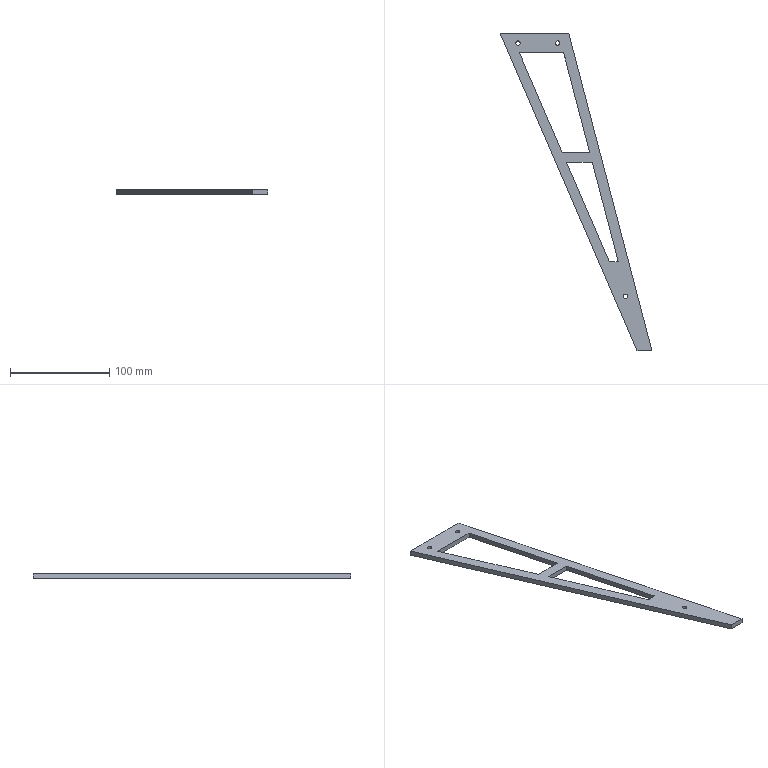Part | SolidWorks | features ICE 3, Extrusion 1 | 1 solid | 20 faces | box 152.846 x 320 x 5 mm | volume 40320 mm3 | plane 14 | cylinder 6 | commonest cylinder face diameters 4.4 x6
STEP:
#1=CARTESIAN_POINT('',(226.262,-608.,-2.5));
#2=VERTEX_POINT('',#1);
#3=CARTESIAN_POINT('',(230.662,-608.,-2.5));
#4=VERTEX_POINT('',#3);
#5=CARTESIAN_POINT('',(228.462,-608.,-2.5));
#6=DIRECTION('',(0.,0.,1.));
#7=DIRECTION('',(1.,0.,0.));
#8=AXIS2_PLACEMENT_3D('',#5,#6,#7);
#9=CIRCLE('',#8,2.2);
#10=EDGE_CURVE('',#2,#4,#9,.T.);
#11=ORIENTED_EDGE('',*,*,#10,.F.);
#12=CARTESIAN_POINT('',(226.262,-608.,2.5));
#13=VERTEX_POINT('',#12);
#14=CARTESIAN_POINT('',(226.262,-608.,-7.5));
#15=DIRECTION('',(0.,0.,1.));
#16=VECTOR('',#15,1000.);
#17=LINE('',#14,#16);
#18=EDGE_CURVE('',#2,#13,#17,.T.);
#19=ORIENTED_EDGE('',*,*,#18,.T.);
#20=CARTESIAN_POINT('',(230.662,-608.,2.5));
#21=VERTEX_POINT('',#20);
#22=CARTESIAN_POINT('',(228.462,-608.,2.5));
#23=DIRECTION('',(0.,0.,1.));
#24=DIRECTION('',(1.,0.,0.));
#25=AXIS2_PLACEMENT_3D('',#22,#23,#24);
#26=CIRCLE('',#25,2.2);
#27=EDGE_CURVE('',#13,#21,#26,.T.);
#28=ORIENTED_EDGE('',*,*,#27,.T.);
#29=CARTESIAN_POINT('',(230.662,-608.,-7.5));
#30=DIRECTION('',(0.,0.,1.));
#31=VECTOR('',#30,1000.);
#32=LINE('',#29,#31);
#33=EDGE_CURVE('',#4,#21,#32,.T.);
#34=ORIENTED_EDGE('',*,*,#33,.F.);
#35=EDGE_LOOP('',(#11,#19,#28,#34));
#36=FACE_OUTER_BOUND('',#35,.T.);
#37=CARTESIAN_POINT('',(228.462,-608.,-7.5));
#38=DIRECTION('',(0.,0.,1.));
#39=DIRECTION('',(1.,0.,0.));
#40=AXIS2_PLACEMENT_3D('',#37,#38,#39);
#41=CYLINDRICAL_SURFACE('',#40,2.2);
#42=ADVANCED_FACE('',(#36),#41,.F.);
#43=CARTESIAN_POINT('',(117.992,-353.,-2.5));
#44=VERTEX_POINT('',#43);
#45=CARTESIAN_POINT('',(122.392,-353.,-2.5));
#46=VERTEX_POINT('',#45);
#47=CARTESIAN_POINT('',(120.192,-353.,-2.5));
#48=DIRECTION('',(0.,0.,1.));
#49=DIRECTION('',(1.,0.,0.));
#50=AXIS2_PLACEMENT_3D('',#47,#48,#49);
#51=CIRCLE('',#50,2.2);
#52=EDGE_CURVE('',#44,#46,#51,.T.);
#53=ORIENTED_EDGE('',*,*,#52,.F.);
#54=CARTESIAN_POINT('',(117.992,-353.,2.5));
#55=VERTEX_POINT('',#54);
#56=CARTESIAN_POINT('',(117.992,-353.,-7.5));
#57=DIRECTION('',(0.,0.,1.));
#58=VECTOR('',#57,1000.);
#59=LINE('',#56,#58);
#60=EDGE_CURVE('',#44,#55,#59,.T.);
#61=ORIENTED_EDGE('',*,*,#60,.T.);
#62=CARTESIAN_POINT('',(122.392,-353.,2.5));
#63=VERTEX_POINT('',#62);
#64=CARTESIAN_POINT('',(120.192,-353.,2.5));
#65=DIRECTION('',(0.,0.,1.));
#66=DIRECTION('',(1.,0.,0.));
#67=AXIS2_PLACEMENT_3D('',#64,#65,#66);
#68=CIRCLE('',#67,2.2);
#69=EDGE_CURVE('',#55,#63,#68,.T.);
#70=ORIENTED_EDGE('',*,*,#69,.T.);
#71=CARTESIAN_POINT('',(122.392,-353.,-7.5));
#72=DIRECTION('',(0.,0.,1.));
#73=VECTOR('',#72,1000.);
#74=LINE('',#71,#73);
#75=EDGE_CURVE('',#46,#63,#74,.T.);
#76=ORIENTED_EDGE('',*,*,#75,.F.);
#77=EDGE_LOOP('',(#53,#61,#70,#76));
#78=FACE_OUTER_BOUND('',#77,.T.);
#79=CARTESIAN_POINT('',(120.192,-353.,-7.5));
#80=DIRECTION('',(0.,0.,1.));
#81=DIRECTION('',(1.,0.,0.));
#82=AXIS2_PLACEMENT_3D('',#79,#80,#81);
#83=CYLINDRICAL_SURFACE('',#82,2.2);
#84=ADVANCED_FACE('',(#78),#83,.F.);
#85=CARTESIAN_POINT('',(157.992,-353.,-2.5));
#86=VERTEX_POINT('',#85);
#87=CARTESIAN_POINT('',(162.392,-353.,-2.5));
#88=VERTEX_POINT('',#87);
#89=CARTESIAN_POINT('',(160.192,-353.,-2.5));
#90=DIRECTION('',(0.,0.,1.));
#91=DIRECTION('',(1.,0.,0.));
#92=AXIS2_PLACEMENT_3D('',#89,#90,#91);
#93=CIRCLE('',#92,2.2);
#94=EDGE_CURVE('',#86,#88,#93,.T.);
#95=ORIENTED_EDGE('',*,*,#94,.F.);
#96=CARTESIAN_POINT('',(157.992,-353.,2.5));
#97=VERTEX_POINT('',#96);
#98=CARTESIAN_POINT('',(157.992,-353.,-7.5));
#99=DIRECTION('',(0.,0.,1.));
#100=VECTOR('',#99,1000.);
#101=LINE('',#98,#100);
#102=EDGE_CURVE('',#86,#97,#101,.T.);
#103=ORIENTED_EDGE('',*,*,#102,.T.);
#104=CARTESIAN_POINT('',(162.392,-353.,2.5));
#105=VERTEX_POINT('',#104);
#106=CARTESIAN_POINT('',(160.192,-353.,2.5));
#107=DIRECTION('',(0.,0.,1.));
#108=DIRECTION('',(1.,0.,0.));
#109=AXIS2_PLACEMENT_3D('',#106,#107,#108);
#110=CIRCLE('',#109,2.2);
#111=EDGE_CURVE('',#97,#105,#110,.T.);
#112=ORIENTED_EDGE('',*,*,#111,.T.);
#113=CARTESIAN_POINT('',(162.392,-353.,-7.5));
#114=DIRECTION('',(0.,0.,1.));
#115=VECTOR('',#114,1000.);
#116=LINE('',#113,#115);
#117=EDGE_CURVE('',#88,#105,#116,.T.);
#118=ORIENTED_EDGE('',*,*,#117,.F.);
#119=EDGE_LOOP('',(#95,#103,#112,#118));
#120=FACE_OUTER_BOUND('',#119,.T.);
#121=CARTESIAN_POINT('',(160.192,-353.,-7.5));
#122=DIRECTION('',(0.,0.,1.));
#123=DIRECTION('',(1.,0.,0.));
#124=AXIS2_PLACEMENT_3D('',#121,#122,#123);
#125=CYLINDRICAL_SURFACE('',#124,2.2);
#126=ADVANCED_FACE('',(#120),#125,.F.);
#127=CARTESIAN_POINT('',(102.154,-343.,-2.5));
#128=VERTEX_POINT('',#127);
#129=CARTESIAN_POINT('',(171.308,-343.,-2.5));
#130=VERTEX_POINT('',#129);
#131=CARTESIAN_POINT('',(0.,-343.,-2.5));
#132=DIRECTION('',(1.,0.,0.));
#133=VECTOR('',#132,1000.);
#134=LINE('',#131,#133);
#135=EDGE_CURVE('',#128,#130,#134,.T.);
#136=ORIENTED_EDGE('',*,*,#135,.F.);
#137=CARTESIAN_POINT('',(102.154,-343.,2.5));
#138=VERTEX_POINT('',#137);
#139=CARTESIAN_POINT('',(102.154,-343.,2.5));
#140=DIRECTION('',(0.,0.,-1.));
#141=VECTOR('',#140,1000.);
#142=LINE('',#139,#141);
#143=EDGE_CURVE('',#138,#128,#142,.T.);
#144=ORIENTED_EDGE('',*,*,#143,.F.);
#145=CARTESIAN_POINT('',(171.308,-343.,2.5));
#146=VERTEX_POINT('',#145);
#147=CARTESIAN_POINT('',(0.,-343.,2.5));
#148=DIRECTION('',(1.,0.,0.));
#149=VECTOR('',#148,1000.);
#150=LINE('',#147,#149);
#151=EDGE_CURVE('',#138,#146,#150,.T.);
#152=ORIENTED_EDGE('',*,*,#151,.T.);
#153=CARTESIAN_POINT('',(171.308,-343.,2.5));
#154=DIRECTION('',(0.,0.,-1.));
#155=VECTOR('',#154,1000.);
#156=LINE('',#153,#155);
#157=EDGE_CURVE('',#146,#130,#156,.T.);
#158=ORIENTED_EDGE('',*,*,#157,.T.);
#159=EDGE_LOOP('',(#136,#144,#152,#158));
#160=FACE_OUTER_BOUND('',#159,.T.);
#161=CARTESIAN_POINT('',(0.,-343.,2.5));
#162=DIRECTION('',(0.,1.,0.));
#163=DIRECTION('',(0.,0.,1.));
#164=AXIS2_PLACEMENT_3D('',#161,#162,#163);
#165=PLANE('',#164);
#166=ADVANCED_FACE('',(#160),#165,.T.);
#167=CARTESIAN_POINT('',(240.,-663.,-2.5));
#168=VERTEX_POINT('',#167);
#169=CARTESIAN_POINT('',(-38.463,-16.569,-2.5));
#170=DIRECTION('',(-0.3956,0.9184,0.));
#171=VECTOR('',#170,1000.);
#172=LINE('',#169,#171);
#173=EDGE_CURVE('',#168,#128,#172,.T.);
#174=ORIENTED_EDGE('',*,*,#173,.F.);
#175=CARTESIAN_POINT('',(240.,-663.,2.5));
#176=VERTEX_POINT('',#175);
#177=CARTESIAN_POINT('',(240.,-663.,2.5));
#178=DIRECTION('',(0.,0.,-1.));
#179=VECTOR('',#178,1000.);
#180=LINE('',#177,#179);
#181=EDGE_CURVE('',#176,#168,#180,.T.);
#182=ORIENTED_EDGE('',*,*,#181,.F.);
#183=CARTESIAN_POINT('',(-38.463,-16.569,2.5));
#184=DIRECTION('',(-0.3956,0.9184,0.));
#185=VECTOR('',#184,1000.);
#186=LINE('',#183,#185);
#187=EDGE_CURVE('',#176,#138,#186,.T.);
#188=ORIENTED_EDGE('',*,*,#187,.T.);
#189=ORIENTED_EDGE('',*,*,#143,.T.);
#190=EDGE_LOOP('',(#174,#182,#188,#189));
#191=FACE_OUTER_BOUND('',#190,.T.);
#192=CARTESIAN_POINT('',(-38.463,-16.569,2.5));
#193=DIRECTION('',(-0.9184,-0.3956,0.));
#194=DIRECTION('',(0.3956,-0.9184,0.));
#195=AXIS2_PLACEMENT_3D('',#192,#193,#194);
#196=PLANE('',#195);
#197=ADVANCED_FACE('',(#191),#196,.T.);
#198=CARTESIAN_POINT('',(255.,-663.,-2.5));
#199=VERTEX_POINT('',#198);
#200=CARTESIAN_POINT('',(0.,-663.,-2.5));
#201=DIRECTION('',(-1.,0.,0.));
#202=VECTOR('',#201,1000.);
#203=LINE('',#200,#202);
#204=EDGE_CURVE('',#199,#168,#203,.T.);
#205=ORIENTED_EDGE('',*,*,#204,.F.);
#206=CARTESIAN_POINT('',(255.,-663.,2.5));
#207=VERTEX_POINT('',#206);
#208=CARTESIAN_POINT('',(255.,-663.,2.5));
#209=DIRECTION('',(0.,0.,-1.));
#210=VECTOR('',#209,1000.);
#211=LINE('',#208,#210);
#212=EDGE_CURVE('',#207,#199,#211,.T.);
#213=ORIENTED_EDGE('',*,*,#212,.F.);
#214=CARTESIAN_POINT('',(0.,-663.,2.5));
#215=DIRECTION('',(-1.,0.,0.));
#216=VECTOR('',#215,1000.);
#217=LINE('',#214,#216);
#218=EDGE_CURVE('',#207,#176,#217,.T.);
#219=ORIENTED_EDGE('',*,*,#218,.T.);
#220=ORIENTED_EDGE('',*,*,#181,.T.);
#221=EDGE_LOOP('',(#205,#213,#219,#220));
#222=FACE_OUTER_BOUND('',#221,.T.);
#223=CARTESIAN_POINT('',(0.,-663.,2.5));
#224=DIRECTION('',(0.,-1.,0.));
#225=DIRECTION('',(1.,0.,0.));
#226=AXIS2_PLACEMENT_3D('',#223,#224,#225);
#227=PLANE('',#226);
#228=ADVANCED_FACE('',(#222),#227,.T.);
#229=CARTESIAN_POINT('',(76.376,19.975,-2.5));
#230=DIRECTION('',(0.253,-0.9675,0.));
#231=VECTOR('',#230,1000.);
#232=LINE('',#229,#231);
#233=EDGE_CURVE('',#130,#199,#232,.T.);
#234=ORIENTED_EDGE('',*,*,#233,.F.);
#235=ORIENTED_EDGE('',*,*,#157,.F.);
#236=CARTESIAN_POINT('',(76.376,19.975,2.5));
#237=DIRECTION('',(0.253,-0.9675,0.));
#238=VECTOR('',#237,1000.);
#239=LINE('',#236,#238);
#240=EDGE_CURVE('',#146,#207,#239,.T.);
#241=ORIENTED_EDGE('',*,*,#240,.T.);
#242=ORIENTED_EDGE('',*,*,#212,.T.);
#243=EDGE_LOOP('',(#234,#235,#241,#242));
#244=FACE_OUTER_BOUND('',#243,.T.);
#245=CARTESIAN_POINT('',(76.376,19.975,2.5));
#246=DIRECTION('',(0.9675,0.253,0.));
#247=DIRECTION('',(-0.253,0.9675,0.));
#248=AXIS2_PLACEMENT_3D('',#245,#246,#247);
#249=PLANE('',#248);
#250=ADVANCED_FACE('',(#244),#249,.T.);
#251=CARTESIAN_POINT('',(228.462,-608.,2.5));
#252=DIRECTION('',(0.,0.,1.));
#253=DIRECTION('',(1.,0.,0.));
#254=AXIS2_PLACEMENT_3D('',#251,#252,#253);
#255=CIRCLE('',#254,2.2);
#256=EDGE_CURVE('',#21,#13,#255,.T.);
#257=ORIENTED_EDGE('',*,*,#256,.F.);
#258=ORIENTED_EDGE('',*,*,#27,.F.);
#259=EDGE_LOOP('',(#257,#258));
#260=FACE_BOUND('',#259,.T.);
#261=CARTESIAN_POINT('',(164.735,-463.,2.5));
#262=VERTEX_POINT('',#261);
#263=CARTESIAN_POINT('',(192.356,-463.,2.5));
#264=VERTEX_POINT('',#263);
#265=CARTESIAN_POINT('',(0.,-463.,2.5));
#266=DIRECTION('',(1.,0.,0.));
#267=VECTOR('',#266,1000.);
#268=LINE('',#265,#267);
#269=EDGE_CURVE('',#262,#264,#268,.T.);
#270=ORIENTED_EDGE('',*,*,#269,.F.);
#271=CARTESIAN_POINT('',(121.658,-363.,2.5));
#272=VERTEX_POINT('',#271);
#273=CARTESIAN_POINT('',(-29.279,-12.612,2.5));
#274=DIRECTION('',(0.3956,-0.9184,0.));
#275=VECTOR('',#274,1000.);
#276=LINE('',#273,#275);
#277=EDGE_CURVE('',#272,#262,#276,.T.);
#278=ORIENTED_EDGE('',*,*,#277,.F.);
#279=CARTESIAN_POINT('',(166.202,-363.,2.5));
#280=VERTEX_POINT('',#279);
#281=CARTESIAN_POINT('',(0.,-363.,2.5));
#282=DIRECTION('',(1.,0.,0.));
#283=VECTOR('',#282,1000.);
#284=LINE('',#281,#283);
#285=EDGE_CURVE('',#272,#280,#284,.T.);
#286=ORIENTED_EDGE('',*,*,#285,.T.);
#287=CARTESIAN_POINT('',(66.701,17.445,2.5));
#288=DIRECTION('',(-0.253,0.9675,0.));
#289=VECTOR('',#288,1000.);
#290=LINE('',#287,#289);
#291=EDGE_CURVE('',#264,#280,#290,.T.);
#292=ORIENTED_EDGE('',*,*,#291,.F.);
#293=EDGE_LOOP('',(#270,#278,#286,#292));
#294=FACE_BOUND('',#293,.T.);
#295=CARTESIAN_POINT('',(212.119,-573.,2.5));
#296=VERTEX_POINT('',#295);
#297=CARTESIAN_POINT('',(221.125,-573.,2.5));
#298=VERTEX_POINT('',#297);
#299=CARTESIAN_POINT('',(0.,-573.,2.5));
#300=DIRECTION('',(1.,0.,0.));
#301=VECTOR('',#300,1000.);
#302=LINE('',#299,#301);
#303=EDGE_CURVE('',#296,#298,#302,.T.);
#304=ORIENTED_EDGE('',*,*,#303,.F.);
#305=CARTESIAN_POINT('',(169.042,-473.,2.5));
#306=VERTEX_POINT('',#305);
#307=CARTESIAN_POINT('',(-29.279,-12.612,2.5));
#308=DIRECTION('',(0.3956,-0.9184,0.));
#309=VECTOR('',#308,1000.);
#310=LINE('',#307,#309);
#311=EDGE_CURVE('',#306,#296,#310,.T.);
#312=ORIENTED_EDGE('',*,*,#311,.F.);
#313=CARTESIAN_POINT('',(194.971,-473.,2.5));
#314=VERTEX_POINT('',#313);
#315=CARTESIAN_POINT('',(0.,-473.,2.5));
#316=DIRECTION('',(1.,0.,0.));
#317=VECTOR('',#316,1000.);
#318=LINE('',#315,#317);
#319=EDGE_CURVE('',#306,#314,#318,.T.);
#320=ORIENTED_EDGE('',*,*,#319,.T.);
#321=CARTESIAN_POINT('',(66.701,17.445,2.5));
#322=DIRECTION('',(-0.253,0.9675,0.));
#323=VECTOR('',#322,1000.);
#324=LINE('',#321,#323);
#325=EDGE_CURVE('',#298,#314,#324,.T.);
#326=ORIENTED_EDGE('',*,*,#325,.F.);
#327=EDGE_LOOP('',(#304,#312,#320,#326));
#328=FACE_BOUND('',#327,.T.);
#329=CARTESIAN_POINT('',(120.192,-353.,2.5));
#330=DIRECTION('',(0.,0.,1.));
#331=DIRECTION('',(1.,0.,0.));
#332=AXIS2_PLACEMENT_3D('',#329,#330,#331);
#333=CIRCLE('',#332,2.2);
#334=EDGE_CURVE('',#63,#55,#333,.T.);
#335=ORIENTED_EDGE('',*,*,#334,.F.);
#336=ORIENTED_EDGE('',*,*,#69,.F.);
#337=EDGE_LOOP('',(#335,#336));
#338=FACE_BOUND('',#337,.T.);
#339=CARTESIAN_POINT('',(160.192,-353.,2.5));
#340=DIRECTION('',(0.,0.,1.));
#341=DIRECTION('',(1.,0.,0.));
#342=AXIS2_PLACEMENT_3D('',#339,#340,#341);
#343=CIRCLE('',#342,2.2);
#344=EDGE_CURVE('',#105,#97,#343,.T.);
#345=ORIENTED_EDGE('',*,*,#344,.F.);
#346=ORIENTED_EDGE('',*,*,#111,.F.);
#347=EDGE_LOOP('',(#345,#346));
#348=FACE_BOUND('',#347,.T.);
#349=ORIENTED_EDGE('',*,*,#151,.F.);
#350=ORIENTED_EDGE('',*,*,#187,.F.);
#351=ORIENTED_EDGE('',*,*,#218,.F.);
#352=ORIENTED_EDGE('',*,*,#240,.F.);
#353=EDGE_LOOP('',(#349,#350,#351,#352));
#354=FACE_OUTER_BOUND('',#353,.T.);
#355=CARTESIAN_POINT('',(0.,0.,2.5));
#356=DIRECTION('',(0.,0.,1.));
#357=DIRECTION('',(1.,0.,0.));
#358=AXIS2_PLACEMENT_3D('',#355,#356,#357);
#359=PLANE('',#358);
#360=ADVANCED_FACE('',(#260,#294,#328,#338,#348,#354),#359,.T.);
#361=CARTESIAN_POINT('',(228.462,-608.,-2.5));
#362=DIRECTION('',(0.,0.,1.));
#363=DIRECTION('',(1.,0.,0.));
#364=AXIS2_PLACEMENT_3D('',#361,#362,#363);
#365=CIRCLE('',#364,2.2);
#366=EDGE_CURVE('',#4,#2,#365,.T.);
#367=ORIENTED_EDGE('',*,*,#366,.T.);
#368=ORIENTED_EDGE('',*,*,#10,.T.);
#369=EDGE_LOOP('',(#367,#368));
#370=FACE_BOUND('',#369,.T.);
#371=CARTESIAN_POINT('',(121.658,-363.,-2.5));
#372=VERTEX_POINT('',#371);
#373=CARTESIAN_POINT('',(164.735,-463.,-2.5));
#374=VERTEX_POINT('',#373);
#375=CARTESIAN_POINT('',(-29.279,-12.612,-2.5));
#376=DIRECTION('',(0.3956,-0.9184,0.));
#377=VECTOR('',#376,1000.);
#378=LINE('',#375,#377);
#379=EDGE_CURVE('',#372,#374,#378,.T.);
#380=ORIENTED_EDGE('',*,*,#379,.T.);
#381=CARTESIAN_POINT('',(192.356,-463.,-2.5));
#382=VERTEX_POINT('',#381);
#383=CARTESIAN_POINT('',(0.,-463.,-2.5));
#384=DIRECTION('',(1.,0.,0.));
#385=VECTOR('',#384,1000.);
#386=LINE('',#383,#385);
#387=EDGE_CURVE('',#374,#382,#386,.T.);
#388=ORIENTED_EDGE('',*,*,#387,.T.);
#389=CARTESIAN_POINT('',(166.202,-363.,-2.5));
#390=VERTEX_POINT('',#389);
#391=CARTESIAN_POINT('',(66.701,17.445,-2.5));
#392=DIRECTION('',(-0.253,0.9675,0.));
#393=VECTOR('',#392,1000.);
#394=LINE('',#391,#393);
#395=EDGE_CURVE('',#382,#390,#394,.T.);
#396=ORIENTED_EDGE('',*,*,#395,.T.);
#397=CARTESIAN_POINT('',(0.,-363.,-2.5));
#398=DIRECTION('',(1.,0.,0.));
#399=VECTOR('',#398,1000.);
#400=LINE('',#397,#399);
#401=EDGE_CURVE('',#372,#390,#400,.T.);
#402=ORIENTED_EDGE('',*,*,#401,.F.);
#403=EDGE_LOOP('',(#380,#388,#396,#402));
#404=FACE_BOUND('',#403,.T.);
#405=CARTESIAN_POINT('',(169.042,-473.,-2.5));
#406=VERTEX_POINT('',#405);
#407=CARTESIAN_POINT('',(212.119,-573.,-2.5));
#408=VERTEX_POINT('',#407);
#409=CARTESIAN_POINT('',(-29.279,-12.612,-2.5));
#410=DIRECTION('',(0.3956,-0.9184,0.));
#411=VECTOR('',#410,1000.);
#412=LINE('',#409,#411);
#413=EDGE_CURVE('',#406,#408,#412,.T.);
#414=ORIENTED_EDGE('',*,*,#413,.T.);
#415=CARTESIAN_POINT('',(221.125,-573.,-2.5));
#416=VERTEX_POINT('',#415);
#417=CARTESIAN_POINT('',(0.,-573.,-2.5));
#418=DIRECTION('',(1.,0.,0.));
#419=VECTOR('',#418,1000.);
#420=LINE('',#417,#419);
#421=EDGE_CURVE('',#408,#416,#420,.T.);
#422=ORIENTED_EDGE('',*,*,#421,.T.);
#423=CARTESIAN_POINT('',(194.971,-473.,-2.5));
#424=VERTEX_POINT('',#423);
#425=CARTESIAN_POINT('',(66.701,17.445,-2.5));
#426=DIRECTION('',(-0.253,0.9675,0.));
#427=VECTOR('',#426,1000.);
#428=LINE('',#425,#427);
#429=EDGE_CURVE('',#416,#424,#428,.T.);
#430=ORIENTED_EDGE('',*,*,#429,.T.);
#431=CARTESIAN_POINT('',(0.,-473.,-2.5));
#432=DIRECTION('',(1.,0.,0.));
#433=VECTOR('',#432,1000.);
#434=LINE('',#431,#433);
#435=EDGE_CURVE('',#406,#424,#434,.T.);
#436=ORIENTED_EDGE('',*,*,#435,.F.);
#437=EDGE_LOOP('',(#414,#422,#430,#436));
#438=FACE_BOUND('',#437,.T.);
#439=CARTESIAN_POINT('',(120.192,-353.,-2.5));
#440=DIRECTION('',(0.,0.,1.));
#441=DIRECTION('',(1.,0.,0.));
#442=AXIS2_PLACEMENT_3D('',#439,#440,#441);
#443=CIRCLE('',#442,2.2);
#444=EDGE_CURVE('',#46,#44,#443,.T.);
#445=ORIENTED_EDGE('',*,*,#444,.T.);
#446=ORIENTED_EDGE('',*,*,#52,.T.);
#447=EDGE_LOOP('',(#445,#446));
#448=FACE_BOUND('',#447,.T.);
#449=CARTESIAN_POINT('',(160.192,-353.,-2.5));
#450=DIRECTION('',(0.,0.,1.));
#451=DIRECTION('',(1.,0.,0.));
#452=AXIS2_PLACEMENT_3D('',#449,#450,#451);
#453=CIRCLE('',#452,2.2);
#454=EDGE_CURVE('',#88,#86,#453,.T.);
#455=ORIENTED_EDGE('',*,*,#454,.T.);
#456=ORIENTED_EDGE('',*,*,#94,.T.);
#457=EDGE_LOOP('',(#455,#456));
#458=FACE_BOUND('',#457,.T.);
#459=ORIENTED_EDGE('',*,*,#135,.T.);
#460=ORIENTED_EDGE('',*,*,#233,.T.);
#461=ORIENTED_EDGE('',*,*,#204,.T.);
#462=ORIENTED_EDGE('',*,*,#173,.T.);
#463=EDGE_LOOP('',(#459,#460,#461,#462));
#464=FACE_OUTER_BOUND('',#463,.T.);
#465=CARTESIAN_POINT('',(0.,0.,-2.5));
#466=DIRECTION('',(0.,0.,1.));
#467=DIRECTION('',(1.,0.,0.));
#468=AXIS2_PLACEMENT_3D('',#465,#466,#467);
#469=PLANE('',#468);
#470=ADVANCED_FACE('',(#370,#404,#438,#448,#458,#464),#469,.F.);
#471=ORIENTED_EDGE('',*,*,#102,.F.);
#472=ORIENTED_EDGE('',*,*,#454,.F.);
#473=ORIENTED_EDGE('',*,*,#117,.T.);
#474=ORIENTED_EDGE('',*,*,#344,.T.);
#475=EDGE_LOOP('',(#471,#472,#473,#474));
#476=FACE_OUTER_BOUND('',#475,.T.);
#477=CARTESIAN_POINT('',(160.192,-353.,-7.5));
#478=DIRECTION('',(0.,0.,1.));
#479=DIRECTION('',(1.,0.,0.));
#480=AXIS2_PLACEMENT_3D('',#477,#478,#479);
#481=CYLINDRICAL_SURFACE('',#480,2.2);
#482=ADVANCED_FACE('',(#476),#481,.F.);
#483=ORIENTED_EDGE('',*,*,#60,.F.);
#484=ORIENTED_EDGE('',*,*,#444,.F.);
#485=ORIENTED_EDGE('',*,*,#75,.T.);
#486=ORIENTED_EDGE('',*,*,#334,.T.);
#487=EDGE_LOOP('',(#483,#484,#485,#486));
#488=FACE_OUTER_BOUND('',#487,.T.);
#489=CARTESIAN_POINT('',(120.192,-353.,-7.5));
#490=DIRECTION('',(0.,0.,1.));
#491=DIRECTION('',(1.,0.,0.));
#492=AXIS2_PLACEMENT_3D('',#489,#490,#491);
#493=CYLINDRICAL_SURFACE('',#492,2.2);
#494=ADVANCED_FACE('',(#488),#493,.F.);
#495=CARTESIAN_POINT('',(212.119,-573.,-7.5));
#496=DIRECTION('',(0.,0.,1.));
#497=VECTOR('',#496,1000.);
#498=LINE('',#495,#497);
#499=EDGE_CURVE('',#408,#296,#498,.T.);
#500=ORIENTED_EDGE('',*,*,#499,.T.);
#501=ORIENTED_EDGE('',*,*,#303,.T.);
#502=CARTESIAN_POINT('',(221.125,-573.,-7.5));
#503=DIRECTION('',(0.,0.,1.));
#504=VECTOR('',#503,1000.);
#505=LINE('',#502,#504);
#506=EDGE_CURVE('',#416,#298,#505,.T.);
#507=ORIENTED_EDGE('',*,*,#506,.F.);
#508=ORIENTED_EDGE('',*,*,#421,.F.);
#509=EDGE_LOOP('',(#500,#501,#507,#508));
#510=FACE_OUTER_BOUND('',#509,.T.);
#511=CARTESIAN_POINT('',(0.,-573.,-7.5));
#512=DIRECTION('',(0.,-1.,0.));
#513=DIRECTION('',(0.,0.,-1.));
#514=AXIS2_PLACEMENT_3D('',#511,#512,#513);
#515=PLANE('',#514);
#516=ADVANCED_FACE('',(#510),#515,.F.);
#517=CARTESIAN_POINT('',(169.042,-473.,-7.5));
#518=DIRECTION('',(0.,0.,1.));
#519=VECTOR('',#518,1000.);
#520=LINE('',#517,#519);
#521=EDGE_CURVE('',#406,#306,#520,.T.);
#522=ORIENTED_EDGE('',*,*,#521,.T.);
#523=ORIENTED_EDGE('',*,*,#311,.T.);
#524=ORIENTED_EDGE('',*,*,#499,.F.);
#525=ORIENTED_EDGE('',*,*,#413,.F.);
#526=EDGE_LOOP('',(#522,#523,#524,#525));
#527=FACE_OUTER_BOUND('',#526,.T.);
#528=CARTESIAN_POINT('',(-29.279,-12.612,-7.5));
#529=DIRECTION('',(-0.9184,-0.3956,0.));
#530=DIRECTION('',(0.3956,-0.9184,0.));
#531=AXIS2_PLACEMENT_3D('',#528,#529,#530);
#532=PLANE('',#531);
#533=ADVANCED_FACE('',(#527),#532,.F.);
#534=ORIENTED_EDGE('',*,*,#435,.T.);
#535=CARTESIAN_POINT('',(194.971,-473.,-7.5));
#536=DIRECTION('',(0.,0.,1.));
#537=VECTOR('',#536,1000.);
#538=LINE('',#535,#537);
#539=EDGE_CURVE('',#424,#314,#538,.T.);
#540=ORIENTED_EDGE('',*,*,#539,.T.);
#541=ORIENTED_EDGE('',*,*,#319,.F.);
#542=ORIENTED_EDGE('',*,*,#521,.F.);
#543=EDGE_LOOP('',(#534,#540,#541,#542));
#544=FACE_OUTER_BOUND('',#543,.T.);
#545=CARTESIAN_POINT('',(0.,-473.,-7.5));
#546=DIRECTION('',(0.,-1.,0.));
#547=DIRECTION('',(0.,0.,-1.));
#548=AXIS2_PLACEMENT_3D('',#545,#546,#547);
#549=PLANE('',#548);
#550=ADVANCED_FACE('',(#544),#549,.T.);
#551=ORIENTED_EDGE('',*,*,#506,.T.);
#552=ORIENTED_EDGE('',*,*,#325,.T.);
#553=ORIENTED_EDGE('',*,*,#539,.F.);
#554=ORIENTED_EDGE('',*,*,#429,.F.);
#555=EDGE_LOOP('',(#551,#552,#553,#554));
#556=FACE_OUTER_BOUND('',#555,.T.);
#557=CARTESIAN_POINT('',(66.701,17.445,-7.5));
#558=DIRECTION('',(0.9675,0.253,0.));
#559=DIRECTION('',(-0.253,0.9675,0.));
#560=AXIS2_PLACEMENT_3D('',#557,#558,#559);
#561=PLANE('',#560);
#562=ADVANCED_FACE('',(#556),#561,.F.);
#563=CARTESIAN_POINT('',(164.735,-463.,-7.5));
#564=DIRECTION('',(0.,0.,1.));
#565=VECTOR('',#564,1000.);
#566=LINE('',#563,#565);
#567=EDGE_CURVE('',#374,#262,#566,.T.);
#568=ORIENTED_EDGE('',*,*,#567,.T.);
#569=ORIENTED_EDGE('',*,*,#269,.T.);
#570=CARTESIAN_POINT('',(192.356,-463.,-7.5));
#571=DIRECTION('',(0.,0.,1.));
#572=VECTOR('',#571,1000.);
#573=LINE('',#570,#572);
#574=EDGE_CURVE('',#382,#264,#573,.T.);
#575=ORIENTED_EDGE('',*,*,#574,.F.);
#576=ORIENTED_EDGE('',*,*,#387,.F.);
#577=EDGE_LOOP('',(#568,#569,#575,#576));
#578=FACE_OUTER_BOUND('',#577,.T.);
#579=CARTESIAN_POINT('',(0.,-463.,-7.5));
#580=DIRECTION('',(0.,-1.,0.));
#581=DIRECTION('',(1.,0.,0.));
#582=AXIS2_PLACEMENT_3D('',#579,#580,#581);
#583=PLANE('',#582);
#584=ADVANCED_FACE('',(#578),#583,.F.);
#585=CARTESIAN_POINT('',(121.658,-363.,-7.5));
#586=DIRECTION('',(0.,0.,1.));
#587=VECTOR('',#586,1000.);
#588=LINE('',#585,#587);
#589=EDGE_CURVE('',#372,#272,#588,.T.);
#590=ORIENTED_EDGE('',*,*,#589,.T.);
#591=ORIENTED_EDGE('',*,*,#277,.T.);
#592=ORIENTED_EDGE('',*,*,#567,.F.);
#593=ORIENTED_EDGE('',*,*,#379,.F.);
#594=EDGE_LOOP('',(#590,#591,#592,#593));
#595=FACE_OUTER_BOUND('',#594,.T.);
#596=CARTESIAN_POINT('',(-29.279,-12.612,-7.5));
#597=DIRECTION('',(-0.9184,-0.3956,0.));
#598=DIRECTION('',(0.3956,-0.9184,0.));
#599=AXIS2_PLACEMENT_3D('',#596,#597,#598);
#600=PLANE('',#599);
#601=ADVANCED_FACE('',(#595),#600,.F.);
#602=ORIENTED_EDGE('',*,*,#401,.T.);
#603=CARTESIAN_POINT('',(166.202,-363.,-7.5));
#604=DIRECTION('',(0.,0.,1.));
#605=VECTOR('',#604,1000.);
#606=LINE('',#603,#605);
#607=EDGE_CURVE('',#390,#280,#606,.T.);
#608=ORIENTED_EDGE('',*,*,#607,.T.);
#609=ORIENTED_EDGE('',*,*,#285,.F.);
#610=ORIENTED_EDGE('',*,*,#589,.F.);
#611=EDGE_LOOP('',(#602,#608,#609,#610));
#612=FACE_OUTER_BOUND('',#611,.T.);
#613=CARTESIAN_POINT('',(0.,-363.,-7.5));
#614=DIRECTION('',(0.,-1.,0.));
#615=DIRECTION('',(0.,0.,-1.));
#616=AXIS2_PLACEMENT_3D('',#613,#614,#615);
#617=PLANE('',#616);
#618=ADVANCED_FACE('',(#612),#617,.T.);
#619=ORIENTED_EDGE('',*,*,#574,.T.);
#620=ORIENTED_EDGE('',*,*,#291,.T.);
#621=ORIENTED_EDGE('',*,*,#607,.F.);
#622=ORIENTED_EDGE('',*,*,#395,.F.);
#623=EDGE_LOOP('',(#619,#620,#621,#622));
#624=FACE_OUTER_BOUND('',#623,.T.);
#625=CARTESIAN_POINT('',(66.701,17.445,-7.5));
#626=DIRECTION('',(0.9675,0.253,0.));
#627=DIRECTION('',(-0.253,0.9675,0.));
#628=AXIS2_PLACEMENT_3D('',#625,#626,#627);
#629=PLANE('',#628);
#630=ADVANCED_FACE('',(#624),#629,.F.);
#631=ORIENTED_EDGE('',*,*,#18,.F.);
#632=ORIENTED_EDGE('',*,*,#366,.F.);
#633=ORIENTED_EDGE('',*,*,#33,.T.);
#634=ORIENTED_EDGE('',*,*,#256,.T.);
#635=EDGE_LOOP('',(#631,#632,#633,#634));
#636=FACE_OUTER_BOUND('',#635,.T.);
#637=CARTESIAN_POINT('',(228.462,-608.,-7.5));
#638=DIRECTION('',(0.,0.,1.));
#639=DIRECTION('',(1.,0.,0.));
#640=AXIS2_PLACEMENT_3D('',#637,#638,#639);
#641=CYLINDRICAL_SURFACE('',#640,2.2);
#642=ADVANCED_FACE('',(#636),#641,.F.);
#643=CLOSED_SHELL('',(#42,#84,#126,#166,#197,#228,#250,#360,#470,#482,#494,#516,#533,#550,#562,#584,#601,#618,#630,#642));
#644=MANIFOLD_SOLID_BREP('',#643);
#645=CARTESIAN_POINT('',(0.,0.,0.));
#646=DIRECTION('',(0.,0.,1.));
#647=DIRECTION('',(1.,0.,0.));
#648=AXIS2_PLACEMENT_3D('',#645,#646,#647);
#649=(LENGTH_UNIT()NAMED_UNIT(*)SI_UNIT(.MILLI.,.METRE.));
#650=UNCERTAINTY_MEASURE_WITH_UNIT(LENGTH_MEASURE(0.00001),#649,'','');
#651=(NAMED_UNIT(*)PLANE_ANGLE_UNIT()SI_UNIT($,.RADIAN.));
#652=(NAMED_UNIT(*)SI_UNIT($,.STERADIAN.)SOLID_ANGLE_UNIT());
#653=(GEOMETRIC_REPRESENTATION_CONTEXT(3)GLOBAL_UNCERTAINTY_ASSIGNED_CONTEXT((#650))GLOBAL_UNIT_ASSIGNED_CONTEXT((#649,#651,#652))REPRESENTATION_CONTEXT('',''));
#654=ADVANCED_BREP_SHAPE_REPRESENTATION('',(#644,#648),#653);